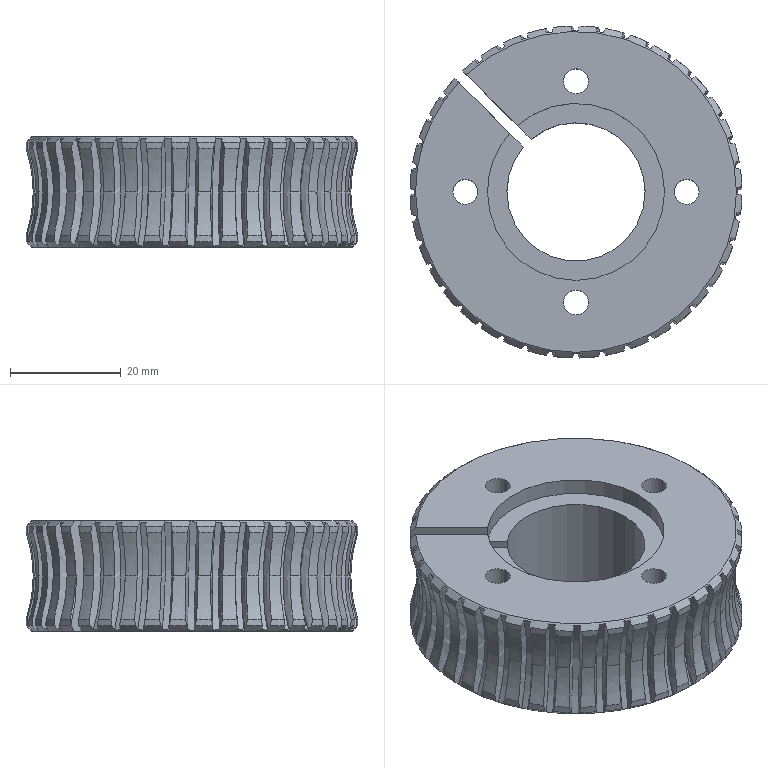Part | SolidWorks | features ICE 2, CirPattern 1, Helix 1, HoleWzd 1, RefAxis 1, Revolution 1, SweepCut 1 | 1 solid | 316 faces | box 60.008 x 60.008 x 20 mm | volume 38918 mm3 | cylinder 141 | torus 80 | spline 80 | plane 9 | cone 6 | commonest cylinder face diameters 60.02 x80 47.7 x39 4.5 x8 8 x8 25 x3 32 x3